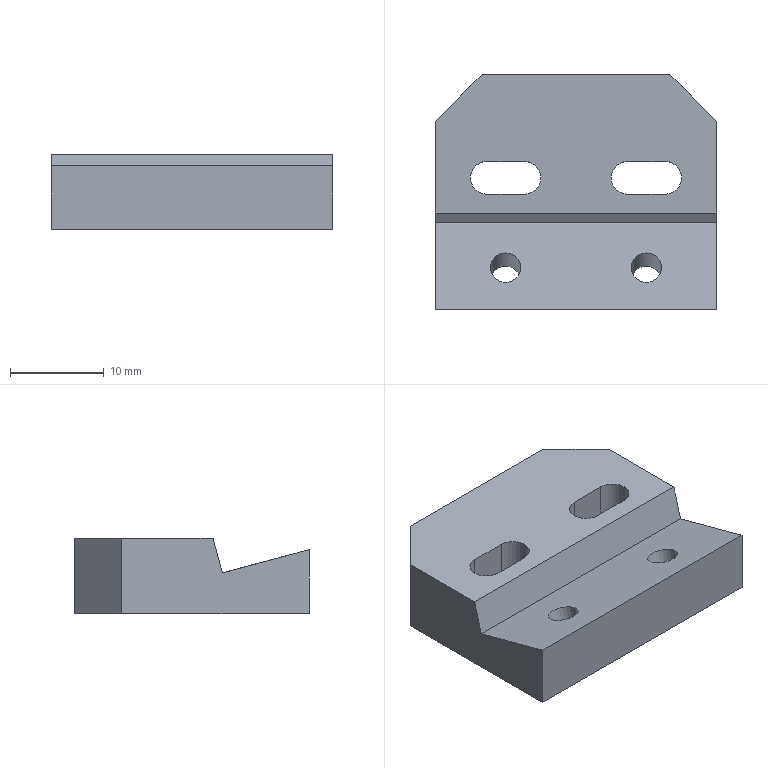Part | NX | 1 solid | 20 faces | box 30 x 25 x 8 mm | volume 4596 mm3 | plane 14 | cylinder 6 | commonest cylinder face diameters 3.5 x4 3.242 x2
STEP:
#1=CARTESIAN_POINT('',(10.,12.5,0.));
#2=VERTEX_POINT('',#1);
#3=CARTESIAN_POINT('',(15.,7.5,0.));
#4=VERTEX_POINT('',#3);
#5=CARTESIAN_POINT('',(12.5,10.,0.));
#6=DIRECTION('',(0.7071,-0.7071,0.));
#7=VECTOR('',#6,1000.);
#8=LINE('',#5,#7);
#9=EDGE_CURVE('',#2,#4,#8,.T.);
#10=ORIENTED_EDGE('',*,*,#9,.T.);
#11=CARTESIAN_POINT('',(15.,7.5,-8.));
#12=VERTEX_POINT('',#11);
#13=CARTESIAN_POINT('',(15.,7.5,-4.));
#14=DIRECTION('',(0.,0.,1.));
#15=VECTOR('',#14,1000.);
#16=LINE('',#13,#15);
#17=EDGE_CURVE('',#12,#4,#16,.T.);
#18=ORIENTED_EDGE('',*,*,#17,.F.);
#19=CARTESIAN_POINT('',(10.,12.5,-8.));
#20=VERTEX_POINT('',#19);
#21=CARTESIAN_POINT('',(12.5,10.,-8.));
#22=DIRECTION('',(0.7071,-0.7071,0.));
#23=VECTOR('',#22,1000.);
#24=LINE('',#21,#23);
#25=EDGE_CURVE('',#20,#12,#24,.T.);
#26=ORIENTED_EDGE('',*,*,#25,.F.);
#27=CARTESIAN_POINT('',(10.,12.5,-4.));
#28=DIRECTION('',(0.,0.,1.));
#29=VECTOR('',#28,1000.);
#30=LINE('',#27,#29);
#31=EDGE_CURVE('',#20,#2,#30,.T.);
#32=ORIENTED_EDGE('',*,*,#31,.T.);
#33=EDGE_LOOP('',(#10,#18,#26,#32));
#34=FACE_BOUND('',#33,.T.);
#35=CARTESIAN_POINT('',(10.,12.5,-4.));
#36=DIRECTION('',(0.7071,0.7071,0.));
#37=DIRECTION('',(0.,0.,1.));
#38=AXIS2_PLACEMENT_3D('',#35,#36,#37);
#39=PLANE('',#38);
#40=ADVANCED_FACE('',(#34),#39,.T.);
#41=ORIENTED_EDGE('',*,*,#31,.F.);
#42=CARTESIAN_POINT('',(-10.,12.5,-8.));
#43=VERTEX_POINT('',#42);
#44=CARTESIAN_POINT('',(0.,12.5,-8.));
#45=DIRECTION('',(1.,0.,0.));
#46=VECTOR('',#45,1000.);
#47=LINE('',#44,#46);
#48=EDGE_CURVE('',#43,#20,#47,.T.);
#49=ORIENTED_EDGE('',*,*,#48,.F.);
#50=CARTESIAN_POINT('',(-10.,12.5,0.));
#51=VERTEX_POINT('',#50);
#52=CARTESIAN_POINT('',(-10.,12.5,-4.));
#53=DIRECTION('',(0.,0.,1.));
#54=VECTOR('',#53,1000.);
#55=LINE('',#52,#54);
#56=EDGE_CURVE('',#43,#51,#55,.T.);
#57=ORIENTED_EDGE('',*,*,#56,.T.);
#58=CARTESIAN_POINT('',(0.,12.5,0.));
#59=DIRECTION('',(1.,0.,0.));
#60=VECTOR('',#59,1000.);
#61=LINE('',#58,#60);
#62=EDGE_CURVE('',#51,#2,#61,.T.);
#63=ORIENTED_EDGE('',*,*,#62,.T.);
#64=EDGE_LOOP('',(#41,#49,#57,#63));
#65=FACE_BOUND('',#64,.T.);
#66=CARTESIAN_POINT('',(-15.,12.5,-8.));
#67=DIRECTION('',(0.,-1.,0.));
#68=DIRECTION('',(1.,0.,0.));
#69=AXIS2_PLACEMENT_3D('',#66,#67,#68);
#70=PLANE('',#69);
#71=ADVANCED_FACE('',(#65),#70,.F.);
#72=CARTESIAN_POINT('',(-9.5,3.25,0.));
#73=VERTEX_POINT('',#72);
#74=CARTESIAN_POINT('',(-9.5,-0.25,0.));
#75=VERTEX_POINT('',#74);
#76=CARTESIAN_POINT('',(-9.5,1.5,0.));
#77=DIRECTION('',(0.,0.,1.));
#78=DIRECTION('',(-1.,0.,0.));
#79=AXIS2_PLACEMENT_3D('',#76,#77,#78);
#80=CIRCLE('',#79,1.75);
#81=EDGE_CURVE('',#73,#75,#80,.T.);
#82=ORIENTED_EDGE('',*,*,#81,.F.);
#83=CARTESIAN_POINT('',(-5.5,3.25,0.));
#84=VERTEX_POINT('',#83);
#85=CARTESIAN_POINT('',(-7.5,3.25,0.));
#86=DIRECTION('',(1.,0.,0.));
#87=VECTOR('',#86,1000.);
#88=LINE('',#85,#87);
#89=EDGE_CURVE('',#73,#84,#88,.T.);
#90=ORIENTED_EDGE('',*,*,#89,.T.);
#91=CARTESIAN_POINT('',(-5.5,-0.25,0.));
#92=VERTEX_POINT('',#91);
#93=CARTESIAN_POINT('',(-5.5,1.5,0.));
#94=DIRECTION('',(0.,0.,1.));
#95=DIRECTION('',(-1.,0.,0.));
#96=AXIS2_PLACEMENT_3D('',#93,#94,#95);
#97=CIRCLE('',#96,1.75);
#98=EDGE_CURVE('',#92,#84,#97,.T.);
#99=ORIENTED_EDGE('',*,*,#98,.F.);
#100=CARTESIAN_POINT('',(-7.5,-0.25,0.));
#101=DIRECTION('',(-1.,0.,0.));
#102=VECTOR('',#101,1000.);
#103=LINE('',#100,#102);
#104=EDGE_CURVE('',#92,#75,#103,.T.);
#105=ORIENTED_EDGE('',*,*,#104,.T.);
#106=EDGE_LOOP('',(#82,#90,#99,#105));
#107=FACE_BOUND('',#106,.T.);
#108=CARTESIAN_POINT('',(5.5,3.25,0.));
#109=VERTEX_POINT('',#108);
#110=CARTESIAN_POINT('',(5.5,-0.25,0.));
#111=VERTEX_POINT('',#110);
#112=CARTESIAN_POINT('',(5.5,1.5,0.));
#113=DIRECTION('',(0.,0.,1.));
#114=DIRECTION('',(-1.,0.,0.));
#115=AXIS2_PLACEMENT_3D('',#112,#113,#114);
#116=CIRCLE('',#115,1.75);
#117=EDGE_CURVE('',#109,#111,#116,.T.);
#118=ORIENTED_EDGE('',*,*,#117,.F.);
#119=CARTESIAN_POINT('',(9.5,3.25,0.));
#120=VERTEX_POINT('',#119);
#121=CARTESIAN_POINT('',(7.5,3.25,0.));
#122=DIRECTION('',(1.,0.,0.));
#123=VECTOR('',#122,1000.);
#124=LINE('',#121,#123);
#125=EDGE_CURVE('',#109,#120,#124,.T.);
#126=ORIENTED_EDGE('',*,*,#125,.T.);
#127=CARTESIAN_POINT('',(9.5,-0.25,0.));
#128=VERTEX_POINT('',#127);
#129=CARTESIAN_POINT('',(9.5,1.5,0.));
#130=DIRECTION('',(0.,0.,1.));
#131=DIRECTION('',(-1.,0.,0.));
#132=AXIS2_PLACEMENT_3D('',#129,#130,#131);
#133=CIRCLE('',#132,1.75);
#134=EDGE_CURVE('',#128,#120,#133,.T.);
#135=ORIENTED_EDGE('',*,*,#134,.F.);
#136=CARTESIAN_POINT('',(7.5,-0.25,0.));
#137=DIRECTION('',(-1.,0.,0.));
#138=VECTOR('',#137,1000.);
#139=LINE('',#136,#138);
#140=EDGE_CURVE('',#128,#111,#139,.T.);
#141=ORIENTED_EDGE('',*,*,#140,.T.);
#142=EDGE_LOOP('',(#118,#126,#135,#141));
#143=FACE_BOUND('',#142,.T.);
#144=ORIENTED_EDGE('',*,*,#62,.F.);
#145=CARTESIAN_POINT('',(-15.,7.5,0.));
#146=VERTEX_POINT('',#145);
#147=CARTESIAN_POINT('',(-12.5,10.,0.));
#148=DIRECTION('',(0.7071,0.7071,0.));
#149=VECTOR('',#148,1000.);
#150=LINE('',#147,#149);
#151=EDGE_CURVE('',#146,#51,#150,.T.);
#152=ORIENTED_EDGE('',*,*,#151,.F.);
#153=CARTESIAN_POINT('',(-15.,-2.244,0.));
#154=VERTEX_POINT('',#153);
#155=CARTESIAN_POINT('',(-15.,2.628,0.));
#156=DIRECTION('',(0.,1.,0.));
#157=VECTOR('',#156,1000.);
#158=LINE('',#155,#157);
#159=EDGE_CURVE('',#154,#146,#158,.T.);
#160=ORIENTED_EDGE('',*,*,#159,.F.);
#161=CARTESIAN_POINT('',(15.,-2.244,0.));
#162=VERTEX_POINT('',#161);
#163=CARTESIAN_POINT('',(0.,-2.244,0.));
#164=DIRECTION('',(-1.,0.,0.));
#165=VECTOR('',#164,1000.);
#166=LINE('',#163,#165);
#167=EDGE_CURVE('',#162,#154,#166,.T.);
#168=ORIENTED_EDGE('',*,*,#167,.F.);
#169=CARTESIAN_POINT('',(15.,2.628,0.));
#170=DIRECTION('',(0.,-1.,0.));
#171=VECTOR('',#170,1000.);
#172=LINE('',#169,#171);
#173=EDGE_CURVE('',#4,#162,#172,.T.);
#174=ORIENTED_EDGE('',*,*,#173,.F.);
#175=ORIENTED_EDGE('',*,*,#9,.F.);
#176=EDGE_LOOP('',(#144,#152,#160,#168,#174,#175));
#177=FACE_BOUND('',#176,.T.);
#178=CARTESIAN_POINT('',(0.,0.,0.));
#179=DIRECTION('',(0.,0.,1.));
#180=DIRECTION('',(0.,-1.,0.));
#181=AXIS2_PLACEMENT_3D('',#178,#179,#180);
#182=PLANE('',#181);
#183=ADVANCED_FACE('',(#107,#143,#177),#182,.T.);
#184=CARTESIAN_POINT('',(-5.5,-0.25,-8.));
#185=VERTEX_POINT('',#184);
#186=CARTESIAN_POINT('',(-9.5,-0.25,-8.));
#187=VERTEX_POINT('',#186);
#188=CARTESIAN_POINT('',(-7.5,-0.25,-8.));
#189=DIRECTION('',(-1.,0.,0.));
#190=VECTOR('',#189,1000.);
#191=LINE('',#188,#190);
#192=EDGE_CURVE('',#185,#187,#191,.T.);
#193=ORIENTED_EDGE('',*,*,#192,.F.);
#194=CARTESIAN_POINT('',(-5.5,3.25,-8.));
#195=VERTEX_POINT('',#194);
#196=CARTESIAN_POINT('',(-5.5,1.5,-8.));
#197=DIRECTION('',(0.,0.,1.));
#198=DIRECTION('',(-1.,0.,0.));
#199=AXIS2_PLACEMENT_3D('',#196,#197,#198);
#200=CIRCLE('',#199,1.75);
#201=EDGE_CURVE('',#185,#195,#200,.T.);
#202=ORIENTED_EDGE('',*,*,#201,.T.);
#203=CARTESIAN_POINT('',(-9.5,3.25,-8.));
#204=VERTEX_POINT('',#203);
#205=CARTESIAN_POINT('',(-7.5,3.25,-8.));
#206=DIRECTION('',(1.,0.,0.));
#207=VECTOR('',#206,1000.);
#208=LINE('',#205,#207);
#209=EDGE_CURVE('',#204,#195,#208,.T.);
#210=ORIENTED_EDGE('',*,*,#209,.F.);
#211=CARTESIAN_POINT('',(-9.5,1.5,-8.));
#212=DIRECTION('',(0.,0.,1.));
#213=DIRECTION('',(-1.,0.,0.));
#214=AXIS2_PLACEMENT_3D('',#211,#212,#213);
#215=CIRCLE('',#214,1.75);
#216=EDGE_CURVE('',#204,#187,#215,.T.);
#217=ORIENTED_EDGE('',*,*,#216,.T.);
#218=EDGE_LOOP('',(#193,#202,#210,#217));
#219=FACE_BOUND('',#218,.T.);
#220=CARTESIAN_POINT('',(9.5,-0.25,-8.));
#221=VERTEX_POINT('',#220);
#222=CARTESIAN_POINT('',(5.5,-0.25,-8.));
#223=VERTEX_POINT('',#222);
#224=CARTESIAN_POINT('',(7.5,-0.25,-8.));
#225=DIRECTION('',(-1.,0.,0.));
#226=VECTOR('',#225,1000.);
#227=LINE('',#224,#226);
#228=EDGE_CURVE('',#221,#223,#227,.T.);
#229=ORIENTED_EDGE('',*,*,#228,.F.);
#230=CARTESIAN_POINT('',(9.5,3.25,-8.));
#231=VERTEX_POINT('',#230);
#232=CARTESIAN_POINT('',(9.5,1.5,-8.));
#233=DIRECTION('',(0.,0.,1.));
#234=DIRECTION('',(-1.,0.,0.));
#235=AXIS2_PLACEMENT_3D('',#232,#233,#234);
#236=CIRCLE('',#235,1.75);
#237=EDGE_CURVE('',#221,#231,#236,.T.);
#238=ORIENTED_EDGE('',*,*,#237,.T.);
#239=CARTESIAN_POINT('',(5.5,3.25,-8.));
#240=VERTEX_POINT('',#239);
#241=CARTESIAN_POINT('',(7.5,3.25,-8.));
#242=DIRECTION('',(1.,0.,0.));
#243=VECTOR('',#242,1000.);
#244=LINE('',#241,#243);
#245=EDGE_CURVE('',#240,#231,#244,.T.);
#246=ORIENTED_EDGE('',*,*,#245,.F.);
#247=CARTESIAN_POINT('',(5.5,1.5,-8.));
#248=DIRECTION('',(0.,0.,1.));
#249=DIRECTION('',(-1.,0.,0.));
#250=AXIS2_PLACEMENT_3D('',#247,#248,#249);
#251=CIRCLE('',#250,1.75);
#252=EDGE_CURVE('',#240,#223,#251,.T.);
#253=ORIENTED_EDGE('',*,*,#252,.T.);
#254=EDGE_LOOP('',(#229,#238,#246,#253));
#255=FACE_BOUND('',#254,.T.);
#256=CARTESIAN_POINT('',(7.5,-11.242,-8.));
#257=VERTEX_POINT('',#256);
#258=CARTESIAN_POINT('',(7.5,-9.564,-8.));
#259=DIRECTION('',(0.,0.,1.));
#260=DIRECTION('',(0.,-1.,0.));
#261=AXIS2_PLACEMENT_3D('',#258,#259,#260);
#262=ELLIPSE('',#261,1.678,1.621);
#263=EDGE_CURVE('',#257,#257,#262,.F.);
#264=ORIENTED_EDGE('',*,*,#263,.F.);
#265=EDGE_LOOP('',(#264));
#266=FACE_BOUND('',#265,.T.);
#267=CARTESIAN_POINT('',(-7.5,-11.242,-8.));
#268=VERTEX_POINT('',#267);
#269=CARTESIAN_POINT('',(-7.5,-9.564,-8.));
#270=DIRECTION('',(0.,0.,1.));
#271=DIRECTION('',(0.,-1.,0.));
#272=AXIS2_PLACEMENT_3D('',#269,#270,#271);
#273=ELLIPSE('',#272,1.678,1.621);
#274=EDGE_CURVE('',#268,#268,#273,.F.);
#275=ORIENTED_EDGE('',*,*,#274,.F.);
#276=EDGE_LOOP('',(#275));
#277=FACE_BOUND('',#276,.T.);
#278=ORIENTED_EDGE('',*,*,#25,.T.);
#279=CARTESIAN_POINT('',(15.,-12.5,-8.));
#280=VERTEX_POINT('',#279);
#281=CARTESIAN_POINT('',(15.,-2.5,-8.));
#282=DIRECTION('',(0.,-1.,0.));
#283=VECTOR('',#282,1000.);
#284=LINE('',#281,#283);
#285=EDGE_CURVE('',#12,#280,#284,.T.);
#286=ORIENTED_EDGE('',*,*,#285,.T.);
#287=CARTESIAN_POINT('',(-15.,-12.5,-8.));
#288=VERTEX_POINT('',#287);
#289=CARTESIAN_POINT('',(0.,-12.5,-8.));
#290=DIRECTION('',(-1.,0.,0.));
#291=VECTOR('',#290,1000.);
#292=LINE('',#289,#291);
#293=EDGE_CURVE('',#280,#288,#292,.T.);
#294=ORIENTED_EDGE('',*,*,#293,.T.);
#295=CARTESIAN_POINT('',(-15.,7.5,-8.));
#296=VERTEX_POINT('',#295);
#297=CARTESIAN_POINT('',(-15.,-2.5,-8.));
#298=DIRECTION('',(0.,1.,0.));
#299=VECTOR('',#298,1000.);
#300=LINE('',#297,#299);
#301=EDGE_CURVE('',#288,#296,#300,.T.);
#302=ORIENTED_EDGE('',*,*,#301,.T.);
#303=CARTESIAN_POINT('',(-12.5,10.,-8.));
#304=DIRECTION('',(0.7071,0.7071,0.));
#305=VECTOR('',#304,1000.);
#306=LINE('',#303,#305);
#307=EDGE_CURVE('',#296,#43,#306,.T.);
#308=ORIENTED_EDGE('',*,*,#307,.T.);
#309=ORIENTED_EDGE('',*,*,#48,.T.);
#310=EDGE_LOOP('',(#278,#286,#294,#302,#308,#309));
#311=FACE_BOUND('',#310,.T.);
#312=CARTESIAN_POINT('',(0.,0.,-8.));
#313=DIRECTION('',(0.,0.,1.));
#314=DIRECTION('',(0.,-1.,0.));
#315=AXIS2_PLACEMENT_3D('',#312,#313,#314);
#316=PLANE('',#315);
#317=ADVANCED_FACE('',(#219,#255,#266,#277,#311),#316,.F.);
#318=ORIENTED_EDGE('',*,*,#17,.T.);
#319=ORIENTED_EDGE('',*,*,#173,.T.);
#320=CARTESIAN_POINT('',(15.,-3.227,-3.671));
#321=VERTEX_POINT('',#320);
#322=CARTESIAN_POINT('',(15.,-2.735,-1.835));
#323=DIRECTION('',(0.,0.2588,0.9659));
#324=VECTOR('',#323,1000.);
#325=LINE('',#322,#324);
#326=EDGE_CURVE('',#321,#162,#325,.T.);
#327=ORIENTED_EDGE('',*,*,#326,.F.);
#328=CARTESIAN_POINT('',(15.,-12.5,-1.186));
#329=VERTEX_POINT('',#328);
#330=CARTESIAN_POINT('',(15.,-7.864,-2.428));
#331=DIRECTION('',(0.,0.9659,-0.2588));
#332=VECTOR('',#331,1000.);
#333=LINE('',#330,#332);
#334=EDGE_CURVE('',#329,#321,#333,.T.);
#335=ORIENTED_EDGE('',*,*,#334,.F.);
#336=CARTESIAN_POINT('',(15.,-12.5,-4.593));
#337=DIRECTION('',(0.,0.,1.));
#338=VECTOR('',#337,1000.);
#339=LINE('',#336,#338);
#340=EDGE_CURVE('',#280,#329,#339,.T.);
#341=ORIENTED_EDGE('',*,*,#340,.F.);
#342=ORIENTED_EDGE('',*,*,#285,.F.);
#343=EDGE_LOOP('',(#318,#319,#327,#335,#341,#342));
#344=FACE_BOUND('',#343,.T.);
#345=CARTESIAN_POINT('',(15.,12.5,-8.));
#346=DIRECTION('',(-1.,0.,0.));
#347=DIRECTION('',(0.,-1.,0.));
#348=AXIS2_PLACEMENT_3D('',#345,#346,#347);
#349=PLANE('',#348);
#350=ADVANCED_FACE('',(#344),#349,.F.);
#351=ORIENTED_EDGE('',*,*,#151,.T.);
#352=ORIENTED_EDGE('',*,*,#56,.F.);
#353=ORIENTED_EDGE('',*,*,#307,.F.);
#354=CARTESIAN_POINT('',(-15.,7.5,-4.));
#355=DIRECTION('',(0.,0.,1.));
#356=VECTOR('',#355,1000.);
#357=LINE('',#354,#356);
#358=EDGE_CURVE('',#296,#146,#357,.T.);
#359=ORIENTED_EDGE('',*,*,#358,.T.);
#360=EDGE_LOOP('',(#351,#352,#353,#359));
#361=FACE_BOUND('',#360,.T.);
#362=CARTESIAN_POINT('',(-15.,7.5,-4.));
#363=DIRECTION('',(-0.7071,0.7071,0.));
#364=DIRECTION('',(0.,0.,1.));
#365=AXIS2_PLACEMENT_3D('',#362,#363,#364);
#366=PLANE('',#365);
#367=ADVANCED_FACE('',(#361),#366,.T.);
#368=ORIENTED_EDGE('',*,*,#358,.F.);
#369=ORIENTED_EDGE('',*,*,#301,.F.);
#370=CARTESIAN_POINT('',(-15.,-12.5,-1.186));
#371=VERTEX_POINT('',#370);
#372=CARTESIAN_POINT('',(-15.,-12.5,-4.593));
#373=DIRECTION('',(0.,0.,1.));
#374=VECTOR('',#373,1000.);
#375=LINE('',#372,#374);
#376=EDGE_CURVE('',#288,#371,#375,.T.);
#377=ORIENTED_EDGE('',*,*,#376,.T.);
#378=CARTESIAN_POINT('',(-15.,-3.227,-3.671));
#379=VERTEX_POINT('',#378);
#380=CARTESIAN_POINT('',(-15.,-7.864,-2.428));
#381=DIRECTION('',(0.,-0.9659,0.2588));
#382=VECTOR('',#381,1000.);
#383=LINE('',#380,#382);
#384=EDGE_CURVE('',#379,#371,#383,.T.);
#385=ORIENTED_EDGE('',*,*,#384,.F.);
#386=CARTESIAN_POINT('',(-15.,-2.735,-1.835));
#387=DIRECTION('',(0.,-0.2588,-0.9659));
#388=VECTOR('',#387,1000.);
#389=LINE('',#386,#388);
#390=EDGE_CURVE('',#154,#379,#389,.T.);
#391=ORIENTED_EDGE('',*,*,#390,.F.);
#392=ORIENTED_EDGE('',*,*,#159,.T.);
#393=EDGE_LOOP('',(#368,#369,#377,#385,#391,#392));
#394=FACE_BOUND('',#393,.T.);
#395=CARTESIAN_POINT('',(-15.,-12.5,-8.));
#396=DIRECTION('',(1.,0.,0.));
#397=DIRECTION('',(0.,1.,0.));
#398=AXIS2_PLACEMENT_3D('',#395,#396,#397);
#399=PLANE('',#398);
#400=ADVANCED_FACE('',(#394),#399,.F.);
#401=ORIENTED_EDGE('',*,*,#274,.T.);
#402=EDGE_LOOP('',(#401));
#403=FACE_BOUND('',#402,.T.);
#404=CARTESIAN_POINT('',(-7.5,-6.491,-2.796));
#405=VERTEX_POINT('',#404);
#406=CARTESIAN_POINT('',(-7.5,-8.057,-2.376));
#407=DIRECTION('',(0.,0.2588,0.9659));
#408=DIRECTION('',(0.,0.9659,-0.2588));
#409=AXIS2_PLACEMENT_3D('',#406,#407,#408);
#410=CIRCLE('',#409,1.621);
#411=EDGE_CURVE('',#405,#405,#410,.T.);
#412=ORIENTED_EDGE('',*,*,#411,.T.);
#413=EDGE_LOOP('',(#412));
#414=FACE_BOUND('',#413,.T.);
#415=CARTESIAN_POINT('',(-7.5,-8.057,-2.376));
#416=DIRECTION('',(0.,-0.2588,-0.9659));
#417=DIRECTION('',(0.,-0.9659,0.2588));
#418=AXIS2_PLACEMENT_3D('',#415,#416,#417);
#419=CYLINDRICAL_SURFACE('',#418,1.621);
#420=ADVANCED_FACE('',(#403,#414),#419,.F.);
#421=ORIENTED_EDGE('',*,*,#376,.F.);
#422=ORIENTED_EDGE('',*,*,#293,.F.);
#423=ORIENTED_EDGE('',*,*,#340,.T.);
#424=CARTESIAN_POINT('',(0.,-12.5,-1.186));
#425=DIRECTION('',(-1.,0.,0.));
#426=VECTOR('',#425,1000.);
#427=LINE('',#424,#426);
#428=EDGE_CURVE('',#329,#371,#427,.T.);
#429=ORIENTED_EDGE('',*,*,#428,.T.);
#430=EDGE_LOOP('',(#421,#422,#423,#429));
#431=FACE_BOUND('',#430,.T.);
#432=CARTESIAN_POINT('',(15.,-12.5,-8.));
#433=DIRECTION('',(0.,1.,0.));
#434=DIRECTION('',(-1.,0.,0.));
#435=AXIS2_PLACEMENT_3D('',#432,#433,#434);
#436=PLANE('',#435);
#437=ADVANCED_FACE('',(#431),#436,.F.);
#438=CARTESIAN_POINT('',(-9.5,-0.25,-4.));
#439=DIRECTION('',(0.,0.,1.));
#440=VECTOR('',#439,1000.);
#441=LINE('',#438,#440);
#442=EDGE_CURVE('',#187,#75,#441,.T.);
#443=ORIENTED_EDGE('',*,*,#442,.T.);
#444=ORIENTED_EDGE('',*,*,#104,.F.);
#445=CARTESIAN_POINT('',(-5.5,-0.25,-4.));
#446=DIRECTION('',(0.,0.,1.));
#447=VECTOR('',#446,1000.);
#448=LINE('',#445,#447);
#449=EDGE_CURVE('',#185,#92,#448,.T.);
#450=ORIENTED_EDGE('',*,*,#449,.F.);
#451=ORIENTED_EDGE('',*,*,#192,.T.);
#452=EDGE_LOOP('',(#443,#444,#450,#451));
#453=FACE_BOUND('',#452,.T.);
#454=CARTESIAN_POINT('',(9.5,-0.25,0.));
#455=DIRECTION('',(0.,-1.,0.));
#456=DIRECTION('',(-1.,0.,0.));
#457=AXIS2_PLACEMENT_3D('',#454,#455,#456);
#458=PLANE('',#457);
#459=ADVANCED_FACE('',(#453),#458,.F.);
#460=ORIENTED_EDGE('',*,*,#449,.T.);
#461=ORIENTED_EDGE('',*,*,#98,.T.);
#462=CARTESIAN_POINT('',(-5.5,3.25,-4.));
#463=DIRECTION('',(0.,0.,-1.));
#464=VECTOR('',#463,1000.);
#465=LINE('',#462,#464);
#466=EDGE_CURVE('',#84,#195,#465,.T.);
#467=ORIENTED_EDGE('',*,*,#466,.T.);
#468=ORIENTED_EDGE('',*,*,#201,.F.);
#469=EDGE_LOOP('',(#460,#461,#467,#468));
#470=FACE_BOUND('',#469,.T.);
#471=CARTESIAN_POINT('',(-5.5,1.5,-4.));
#472=DIRECTION('',(0.,0.,1.));
#473=DIRECTION('',(0.,-1.,0.));
#474=AXIS2_PLACEMENT_3D('',#471,#472,#473);
#475=CYLINDRICAL_SURFACE('',#474,1.75);
#476=ADVANCED_FACE('',(#470),#475,.F.);
#477=ORIENTED_EDGE('',*,*,#466,.F.);
#478=ORIENTED_EDGE('',*,*,#89,.F.);
#479=CARTESIAN_POINT('',(-9.5,3.25,-4.));
#480=DIRECTION('',(0.,0.,1.));
#481=VECTOR('',#480,1000.);
#482=LINE('',#479,#481);
#483=EDGE_CURVE('',#204,#73,#482,.T.);
#484=ORIENTED_EDGE('',*,*,#483,.F.);
#485=ORIENTED_EDGE('',*,*,#209,.T.);
#486=EDGE_LOOP('',(#477,#478,#484,#485));
#487=FACE_BOUND('',#486,.T.);
#488=CARTESIAN_POINT('',(5.5,3.25,0.));
#489=DIRECTION('',(0.,1.,0.));
#490=DIRECTION('',(1.,0.,0.));
#491=AXIS2_PLACEMENT_3D('',#488,#489,#490);
#492=PLANE('',#491);
#493=ADVANCED_FACE('',(#487),#492,.F.);
#494=ORIENTED_EDGE('',*,*,#483,.T.);
#495=ORIENTED_EDGE('',*,*,#81,.T.);
#496=ORIENTED_EDGE('',*,*,#442,.F.);
#497=ORIENTED_EDGE('',*,*,#216,.F.);
#498=EDGE_LOOP('',(#494,#495,#496,#497));
#499=FACE_BOUND('',#498,.T.);
#500=CARTESIAN_POINT('',(-9.5,1.5,-4.));
#501=DIRECTION('',(0.,0.,1.));
#502=DIRECTION('',(0.,1.,0.));
#503=AXIS2_PLACEMENT_3D('',#500,#501,#502);
#504=CYLINDRICAL_SURFACE('',#503,1.75);
#505=ADVANCED_FACE('',(#499),#504,.F.);
#506=CARTESIAN_POINT('',(5.5,-0.25,-4.));
#507=DIRECTION('',(0.,0.,1.));
#508=VECTOR('',#507,1000.);
#509=LINE('',#506,#508);
#510=EDGE_CURVE('',#223,#111,#509,.T.);
#511=ORIENTED_EDGE('',*,*,#510,.T.);
#512=ORIENTED_EDGE('',*,*,#140,.F.);
#513=CARTESIAN_POINT('',(9.5,-0.25,-4.));
#514=DIRECTION('',(0.,0.,1.));
#515=VECTOR('',#514,1000.);
#516=LINE('',#513,#515);
#517=EDGE_CURVE('',#221,#128,#516,.T.);
#518=ORIENTED_EDGE('',*,*,#517,.F.);
#519=ORIENTED_EDGE('',*,*,#228,.T.);
#520=EDGE_LOOP('',(#511,#512,#518,#519));
#521=FACE_BOUND('',#520,.T.);
#522=CARTESIAN_POINT('',(9.5,-0.25,0.));
#523=DIRECTION('',(0.,-1.,0.));
#524=DIRECTION('',(-1.,0.,0.));
#525=AXIS2_PLACEMENT_3D('',#522,#523,#524);
#526=PLANE('',#525);
#527=ADVANCED_FACE('',(#521),#526,.F.);
#528=ORIENTED_EDGE('',*,*,#517,.T.);
#529=ORIENTED_EDGE('',*,*,#134,.T.);
#530=CARTESIAN_POINT('',(9.5,3.25,-4.));
#531=DIRECTION('',(0.,0.,-1.));
#532=VECTOR('',#531,1000.);
#533=LINE('',#530,#532);
#534=EDGE_CURVE('',#120,#231,#533,.T.);
#535=ORIENTED_EDGE('',*,*,#534,.T.);
#536=ORIENTED_EDGE('',*,*,#237,.F.);
#537=EDGE_LOOP('',(#528,#529,#535,#536));
#538=FACE_BOUND('',#537,.T.);
#539=CARTESIAN_POINT('',(9.5,1.5,-4.));
#540=DIRECTION('',(0.,0.,1.));
#541=DIRECTION('',(0.,-1.,0.));
#542=AXIS2_PLACEMENT_3D('',#539,#540,#541);
#543=CYLINDRICAL_SURFACE('',#542,1.75);
#544=ADVANCED_FACE('',(#538),#543,.F.);
#545=ORIENTED_EDGE('',*,*,#534,.F.);
#546=ORIENTED_EDGE('',*,*,#125,.F.);
#547=CARTESIAN_POINT('',(5.5,3.25,-4.));
#548=DIRECTION('',(0.,0.,1.));
#549=VECTOR('',#548,1000.);
#550=LINE('',#547,#549);
#551=EDGE_CURVE('',#240,#109,#550,.T.);
#552=ORIENTED_EDGE('',*,*,#551,.F.);
#553=ORIENTED_EDGE('',*,*,#245,.T.);
#554=EDGE_LOOP('',(#545,#546,#552,#553));
#555=FACE_BOUND('',#554,.T.);
#556=CARTESIAN_POINT('',(5.5,3.25,0.));
#557=DIRECTION('',(0.,1.,0.));
#558=DIRECTION('',(1.,0.,0.));
#559=AXIS2_PLACEMENT_3D('',#556,#557,#558);
#560=PLANE('',#559);
#561=ADVANCED_FACE('',(#555),#560,.F.);
#562=ORIENTED_EDGE('',*,*,#551,.T.);
#563=ORIENTED_EDGE('',*,*,#117,.T.);
#564=ORIENTED_EDGE('',*,*,#510,.F.);
#565=ORIENTED_EDGE('',*,*,#252,.F.);
#566=EDGE_LOOP('',(#562,#563,#564,#565));
#567=FACE_BOUND('',#566,.T.);
#568=CARTESIAN_POINT('',(5.5,1.5,-4.));
#569=DIRECTION('',(0.,0.,1.));
#570=DIRECTION('',(0.,1.,0.));
#571=AXIS2_PLACEMENT_3D('',#568,#569,#570);
#572=CYLINDRICAL_SURFACE('',#571,1.75);
#573=ADVANCED_FACE('',(#567),#572,.F.);
#574=CARTESIAN_POINT('',(0.,-3.227,-3.671));
#575=DIRECTION('',(-1.,0.,0.));
#576=VECTOR('',#575,1000.);
#577=LINE('',#574,#576);
#578=EDGE_CURVE('',#321,#379,#577,.T.);
#579=ORIENTED_EDGE('',*,*,#578,.F.);
#580=ORIENTED_EDGE('',*,*,#326,.T.);
#581=ORIENTED_EDGE('',*,*,#167,.T.);
#582=ORIENTED_EDGE('',*,*,#390,.T.);
#583=EDGE_LOOP('',(#579,#580,#581,#582));
#584=FACE_BOUND('',#583,.T.);
#585=CARTESIAN_POINT('',(15.,-3.227,-3.671));
#586=DIRECTION('',(0.,-0.9659,0.2588));
#587=DIRECTION('',(0.,0.2588,0.9659));
#588=AXIS2_PLACEMENT_3D('',#585,#586,#587);
#589=PLANE('',#588);
#590=ADVANCED_FACE('',(#584),#589,.T.);
#591=CARTESIAN_POINT('',(7.5,-6.491,-2.796));
#592=VERTEX_POINT('',#591);
#593=CARTESIAN_POINT('',(7.5,-8.057,-2.376));
#594=DIRECTION('',(0.,-0.2588,-0.9659));
#595=DIRECTION('',(0.,0.9659,-0.2588));
#596=AXIS2_PLACEMENT_3D('',#593,#594,#595);
#597=CIRCLE('',#596,1.621);
#598=EDGE_CURVE('',#592,#592,#597,.T.);
#599=ORIENTED_EDGE('',*,*,#598,.T.);
#600=EDGE_LOOP('',(#599));
#601=FACE_BOUND('',#600,.T.);
#602=ORIENTED_EDGE('',*,*,#411,.F.);
#603=EDGE_LOOP('',(#602));
#604=FACE_BOUND('',#603,.T.);
#605=ORIENTED_EDGE('',*,*,#334,.T.);
#606=ORIENTED_EDGE('',*,*,#578,.T.);
#607=ORIENTED_EDGE('',*,*,#384,.T.);
#608=ORIENTED_EDGE('',*,*,#428,.F.);
#609=EDGE_LOOP('',(#605,#606,#607,#608));
#610=FACE_BOUND('',#609,.T.);
#611=CARTESIAN_POINT('',(15.,-16.926,0.));
#612=DIRECTION('',(0.,0.2588,0.9659));
#613=DIRECTION('',(0.,0.9659,-0.2588));
#614=AXIS2_PLACEMENT_3D('',#611,#612,#613);
#615=PLANE('',#614);
#616=ADVANCED_FACE('',(#601,#604,#610),#615,.T.);
#617=ORIENTED_EDGE('',*,*,#263,.T.);
#618=EDGE_LOOP('',(#617));
#619=FACE_BOUND('',#618,.T.);
#620=ORIENTED_EDGE('',*,*,#598,.F.);
#621=EDGE_LOOP('',(#620));
#622=FACE_BOUND('',#621,.T.);
#623=CARTESIAN_POINT('',(7.5,-8.057,-2.376));
#624=DIRECTION('',(0.,-0.2588,-0.9659));
#625=DIRECTION('',(0.,-0.9659,0.2588));
#626=AXIS2_PLACEMENT_3D('',#623,#624,#625);
#627=CYLINDRICAL_SURFACE('',#626,1.621);
#628=ADVANCED_FACE('',(#619,#622),#627,.F.);
#629=CLOSED_SHELL('',(#40,#71,#183,#317,#350,#367,#400,#420,#437,#459,#476,#493,#505,#527,#544,#561,#573,#590,#616,#628));
#630=MANIFOLD_SOLID_BREP('',#629);
#631=(LENGTH_UNIT()NAMED_UNIT(*)SI_UNIT(.MILLI.,.METRE.));
#632=UNCERTAINTY_MEASURE_WITH_UNIT(LENGTH_MEASURE(0.00001),#631,'','');
#633=(NAMED_UNIT(*)PLANE_ANGLE_UNIT()SI_UNIT($,.RADIAN.));
#634=(NAMED_UNIT(*)SI_UNIT($,.STERADIAN.)SOLID_ANGLE_UNIT());
#635=(GEOMETRIC_REPRESENTATION_CONTEXT(3)GLOBAL_UNCERTAINTY_ASSIGNED_CONTEXT((#632))GLOBAL_UNIT_ASSIGNED_CONTEXT((#631,#633,#634))REPRESENTATION_CONTEXT('',''));
#636=ADVANCED_BREP_SHAPE_REPRESENTATION('',(#630),#635);